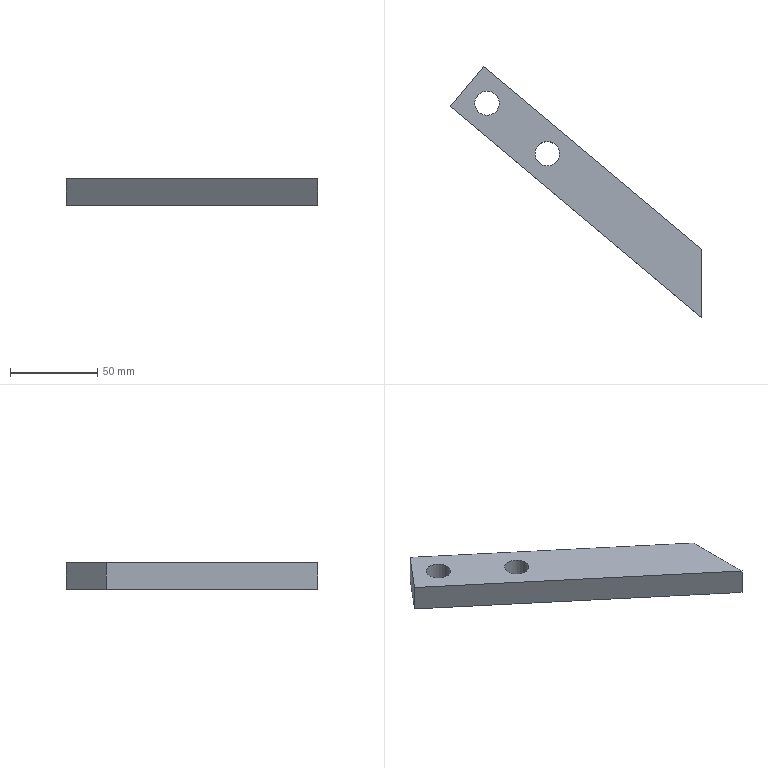Part | NX | features solid 2 | 1 solid | 8 faces | box 144.058 x 143.86 x 15 mm | volume 74342 mm3 | plane 6 | cylinder 2 | commonest cylinder face diameters 14 x2
STEP:
#1=CARTESIAN_POINT('',(-274.791,-28.67,0.));
#2=VERTEX_POINT('',#1);
#3=CARTESIAN_POINT('',(-150.017,-133.368,0.));
#4=VERTEX_POINT('',#3);
#5=CARTESIAN_POINT('',(-274.791,-28.67,0.));
#6=DIRECTION('',(0.766,-0.6428,0.));
#7=VECTOR('',#6,1000.);
#8=LINE('',#5,#7);
#9=EDGE_CURVE('',#2,#4,#8,.T.);
#10=ORIENTED_EDGE('',*,*,#9,.F.);
#11=CARTESIAN_POINT('',(-294.075,-51.651,0.));
#12=VERTEX_POINT('',#11);
#13=CARTESIAN_POINT('',(-294.075,-51.651,0.));
#14=DIRECTION('',(0.6428,0.766,0.));
#15=VECTOR('',#14,1000.);
#16=LINE('',#13,#15);
#17=EDGE_CURVE('',#12,#2,#16,.T.);
#18=ORIENTED_EDGE('',*,*,#17,.F.);
#19=CARTESIAN_POINT('',(-150.017,-172.53,0.));
#20=VERTEX_POINT('',#19);
#21=CARTESIAN_POINT('',(-294.075,-51.651,0.));
#22=DIRECTION('',(0.766,-0.6428,0.));
#23=VECTOR('',#22,1000.);
#24=LINE('',#21,#23);
#25=EDGE_CURVE('',#12,#20,#24,.T.);
#26=ORIENTED_EDGE('',*,*,#25,.T.);
#27=CARTESIAN_POINT('',(-150.017,-51.651,0.));
#28=DIRECTION('',(0.,1.,0.));
#29=VECTOR('',#28,1000.);
#30=LINE('',#27,#29);
#31=EDGE_CURVE('',#20,#4,#30,.T.);
#32=ORIENTED_EDGE('',*,*,#31,.T.);
#33=EDGE_LOOP('',(#10,#18,#26,#32));
#34=FACE_BOUND('',#33,.T.);
#35=CARTESIAN_POINT('',(-265.943,-49.802,0.));
#36=VERTEX_POINT('',#35);
#37=CARTESIAN_POINT('',(-272.943,-49.802,0.));
#38=DIRECTION('',(0.,0.,1.));
#39=DIRECTION('',(1.,0.,0.));
#40=AXIS2_PLACEMENT_3D('',#37,#38,#39);
#41=CIRCLE('',#40,7.);
#42=EDGE_CURVE('',#36,#36,#41,.T.);
#43=ORIENTED_EDGE('',*,*,#42,.F.);
#44=EDGE_LOOP('',(#43));
#45=FACE_BOUND('',#44,.T.);
#46=CARTESIAN_POINT('',(-231.471,-78.728,0.));
#47=VERTEX_POINT('',#46);
#48=CARTESIAN_POINT('',(-238.471,-78.728,0.));
#49=DIRECTION('',(0.,0.,1.));
#50=DIRECTION('',(1.,0.,0.));
#51=AXIS2_PLACEMENT_3D('',#48,#49,#50);
#52=CIRCLE('',#51,7.);
#53=EDGE_CURVE('',#47,#47,#52,.F.);
#54=ORIENTED_EDGE('',*,*,#53,.T.);
#55=EDGE_LOOP('',(#54));
#56=FACE_BOUND('',#55,.T.);
#57=CARTESIAN_POINT('',(-294.075,-51.651,0.));
#58=DIRECTION('',(0.,0.,1.));
#59=DIRECTION('',(1.,0.,0.));
#60=AXIS2_PLACEMENT_3D('',#57,#58,#59);
#61=PLANE('',#60);
#62=ADVANCED_FACE('',(#34,#45,#56),#61,.T.);
#63=CARTESIAN_POINT('',(-274.791,-28.67,-15.));
#64=VERTEX_POINT('',#63);
#65=CARTESIAN_POINT('',(-150.017,-133.368,-15.));
#66=VERTEX_POINT('',#65);
#67=CARTESIAN_POINT('',(-274.791,-28.67,-15.));
#68=DIRECTION('',(0.766,-0.6428,0.));
#69=VECTOR('',#68,1000.);
#70=LINE('',#67,#69);
#71=EDGE_CURVE('',#64,#66,#70,.T.);
#72=ORIENTED_EDGE('',*,*,#71,.T.);
#73=CARTESIAN_POINT('',(-150.017,-172.53,-15.));
#74=VERTEX_POINT('',#73);
#75=CARTESIAN_POINT('',(-150.017,-51.651,-15.));
#76=DIRECTION('',(0.,1.,0.));
#77=VECTOR('',#76,1000.);
#78=LINE('',#75,#77);
#79=EDGE_CURVE('',#74,#66,#78,.T.);
#80=ORIENTED_EDGE('',*,*,#79,.F.);
#81=CARTESIAN_POINT('',(-294.075,-51.651,-15.));
#82=VERTEX_POINT('',#81);
#83=CARTESIAN_POINT('',(-294.075,-51.651,-15.));
#84=DIRECTION('',(0.766,-0.6428,0.));
#85=VECTOR('',#84,1000.);
#86=LINE('',#83,#85);
#87=EDGE_CURVE('',#82,#74,#86,.T.);
#88=ORIENTED_EDGE('',*,*,#87,.F.);
#89=CARTESIAN_POINT('',(-294.075,-51.651,-15.));
#90=DIRECTION('',(0.6428,0.766,0.));
#91=VECTOR('',#90,1000.);
#92=LINE('',#89,#91);
#93=EDGE_CURVE('',#82,#64,#92,.T.);
#94=ORIENTED_EDGE('',*,*,#93,.T.);
#95=EDGE_LOOP('',(#72,#80,#88,#94));
#96=FACE_BOUND('',#95,.T.);
#97=CARTESIAN_POINT('',(-265.943,-49.802,-15.));
#98=VERTEX_POINT('',#97);
#99=CARTESIAN_POINT('',(-272.943,-49.802,-15.));
#100=DIRECTION('',(0.,0.,1.));
#101=DIRECTION('',(1.,0.,0.));
#102=AXIS2_PLACEMENT_3D('',#99,#100,#101);
#103=CIRCLE('',#102,7.);
#104=EDGE_CURVE('',#98,#98,#103,.T.);
#105=ORIENTED_EDGE('',*,*,#104,.T.);
#106=EDGE_LOOP('',(#105));
#107=FACE_BOUND('',#106,.T.);
#108=CARTESIAN_POINT('',(-231.471,-78.728,-15.));
#109=VERTEX_POINT('',#108);
#110=CARTESIAN_POINT('',(-238.471,-78.728,-15.));
#111=DIRECTION('',(0.,0.,1.));
#112=DIRECTION('',(1.,0.,0.));
#113=AXIS2_PLACEMENT_3D('',#110,#111,#112);
#114=CIRCLE('',#113,7.);
#115=EDGE_CURVE('',#109,#109,#114,.F.);
#116=ORIENTED_EDGE('',*,*,#115,.F.);
#117=EDGE_LOOP('',(#116));
#118=FACE_BOUND('',#117,.T.);
#119=CARTESIAN_POINT('',(-294.075,-51.651,-15.));
#120=DIRECTION('',(0.,0.,1.));
#121=DIRECTION('',(1.,0.,0.));
#122=AXIS2_PLACEMENT_3D('',#119,#120,#121);
#123=PLANE('',#122);
#124=ADVANCED_FACE('',(#96,#107,#118),#123,.F.);
#125=CARTESIAN_POINT('',(-294.075,-51.651,-15.));
#126=DIRECTION('',(0.,0.,1.));
#127=VECTOR('',#126,1000.);
#128=LINE('',#125,#127);
#129=EDGE_CURVE('',#82,#12,#128,.T.);
#130=ORIENTED_EDGE('',*,*,#129,.F.);
#131=ORIENTED_EDGE('',*,*,#87,.T.);
#132=CARTESIAN_POINT('',(-150.017,-172.53,-15.));
#133=DIRECTION('',(0.,0.,1.));
#134=VECTOR('',#133,1000.);
#135=LINE('',#132,#134);
#136=EDGE_CURVE('',#74,#20,#135,.T.);
#137=ORIENTED_EDGE('',*,*,#136,.T.);
#138=ORIENTED_EDGE('',*,*,#25,.F.);
#139=EDGE_LOOP('',(#130,#131,#137,#138));
#140=FACE_BOUND('',#139,.T.);
#141=CARTESIAN_POINT('',(-294.075,-51.651,-15.));
#142=DIRECTION('',(-0.6428,-0.766,0.));
#143=DIRECTION('',(0.766,-0.6428,0.));
#144=AXIS2_PLACEMENT_3D('',#141,#142,#143);
#145=PLANE('',#144);
#146=ADVANCED_FACE('',(#140),#145,.T.);
#147=ORIENTED_EDGE('',*,*,#136,.F.);
#148=ORIENTED_EDGE('',*,*,#79,.T.);
#149=CARTESIAN_POINT('',(-150.017,-133.368,0.));
#150=DIRECTION('',(0.,0.,-1.));
#151=VECTOR('',#150,1000.);
#152=LINE('',#149,#151);
#153=EDGE_CURVE('',#66,#4,#152,.F.);
#154=ORIENTED_EDGE('',*,*,#153,.T.);
#155=ORIENTED_EDGE('',*,*,#31,.F.);
#156=EDGE_LOOP('',(#147,#148,#154,#155));
#157=FACE_BOUND('',#156,.T.);
#158=CARTESIAN_POINT('',(-150.017,-164.139,0.));
#159=DIRECTION('',(1.,0.,0.));
#160=DIRECTION('',(0.,0.,-1.));
#161=AXIS2_PLACEMENT_3D('',#158,#159,#160);
#162=PLANE('',#161);
#163=ADVANCED_FACE('',(#157),#162,.T.);
#164=ORIENTED_EDGE('',*,*,#153,.F.);
#165=ORIENTED_EDGE('',*,*,#71,.F.);
#166=CARTESIAN_POINT('',(-274.791,-28.67,-15.));
#167=DIRECTION('',(0.,0.,1.));
#168=VECTOR('',#167,1000.);
#169=LINE('',#166,#168);
#170=EDGE_CURVE('',#64,#2,#169,.T.);
#171=ORIENTED_EDGE('',*,*,#170,.T.);
#172=ORIENTED_EDGE('',*,*,#9,.T.);
#173=EDGE_LOOP('',(#164,#165,#171,#172));
#174=FACE_BOUND('',#173,.T.);
#175=CARTESIAN_POINT('',(-274.791,-28.67,-15.));
#176=DIRECTION('',(-0.6428,-0.766,0.));
#177=DIRECTION('',(0.766,-0.6428,0.));
#178=AXIS2_PLACEMENT_3D('',#175,#176,#177);
#179=PLANE('',#178);
#180=ADVANCED_FACE('',(#174),#179,.F.);
#181=ORIENTED_EDGE('',*,*,#93,.F.);
#182=ORIENTED_EDGE('',*,*,#129,.T.);
#183=ORIENTED_EDGE('',*,*,#17,.T.);
#184=ORIENTED_EDGE('',*,*,#170,.F.);
#185=EDGE_LOOP('',(#181,#182,#183,#184));
#186=FACE_BOUND('',#185,.T.);
#187=CARTESIAN_POINT('',(-294.075,-51.651,-15.));
#188=DIRECTION('',(0.766,-0.6428,0.));
#189=DIRECTION('',(0.6428,0.766,0.));
#190=AXIS2_PLACEMENT_3D('',#187,#188,#189);
#191=PLANE('',#190);
#192=ADVANCED_FACE('',(#186),#191,.F.);
#193=ORIENTED_EDGE('',*,*,#42,.T.);
#194=EDGE_LOOP('',(#193));
#195=FACE_BOUND('',#194,.T.);
#196=ORIENTED_EDGE('',*,*,#104,.F.);
#197=EDGE_LOOP('',(#196));
#198=FACE_BOUND('',#197,.T.);
#199=CARTESIAN_POINT('',(-272.943,-49.802,-215.));
#200=DIRECTION('',(0.,0.,1.));
#201=DIRECTION('',(1.,0.,0.));
#202=AXIS2_PLACEMENT_3D('',#199,#200,#201);
#203=CYLINDRICAL_SURFACE('',#202,7.);
#204=ADVANCED_FACE('',(#195,#198),#203,.F.);
#205=ORIENTED_EDGE('',*,*,#53,.F.);
#206=EDGE_LOOP('',(#205));
#207=FACE_BOUND('',#206,.T.);
#208=ORIENTED_EDGE('',*,*,#115,.T.);
#209=EDGE_LOOP('',(#208));
#210=FACE_BOUND('',#209,.T.);
#211=CARTESIAN_POINT('',(-238.471,-78.728,-215.));
#212=DIRECTION('',(0.,0.,1.));
#213=DIRECTION('',(1.,0.,0.));
#214=AXIS2_PLACEMENT_3D('',#211,#212,#213);
#215=CYLINDRICAL_SURFACE('',#214,7.);
#216=ADVANCED_FACE('',(#207,#210),#215,.F.);
#217=CLOSED_SHELL('',(#62,#124,#146,#163,#180,#192,#204,#216));
#218=MANIFOLD_SOLID_BREP('',#217);
#219=(LENGTH_UNIT()NAMED_UNIT(*)SI_UNIT(.MILLI.,.METRE.));
#220=UNCERTAINTY_MEASURE_WITH_UNIT(LENGTH_MEASURE(0.00001),#219,'','');
#221=(NAMED_UNIT(*)PLANE_ANGLE_UNIT()SI_UNIT($,.RADIAN.));
#222=(NAMED_UNIT(*)SI_UNIT($,.STERADIAN.)SOLID_ANGLE_UNIT());
#223=(GEOMETRIC_REPRESENTATION_CONTEXT(3)GLOBAL_UNCERTAINTY_ASSIGNED_CONTEXT((#220))GLOBAL_UNIT_ASSIGNED_CONTEXT((#219,#221,#222))REPRESENTATION_CONTEXT('',''));
#224=ADVANCED_BREP_SHAPE_REPRESENTATION('',(#218),#223);